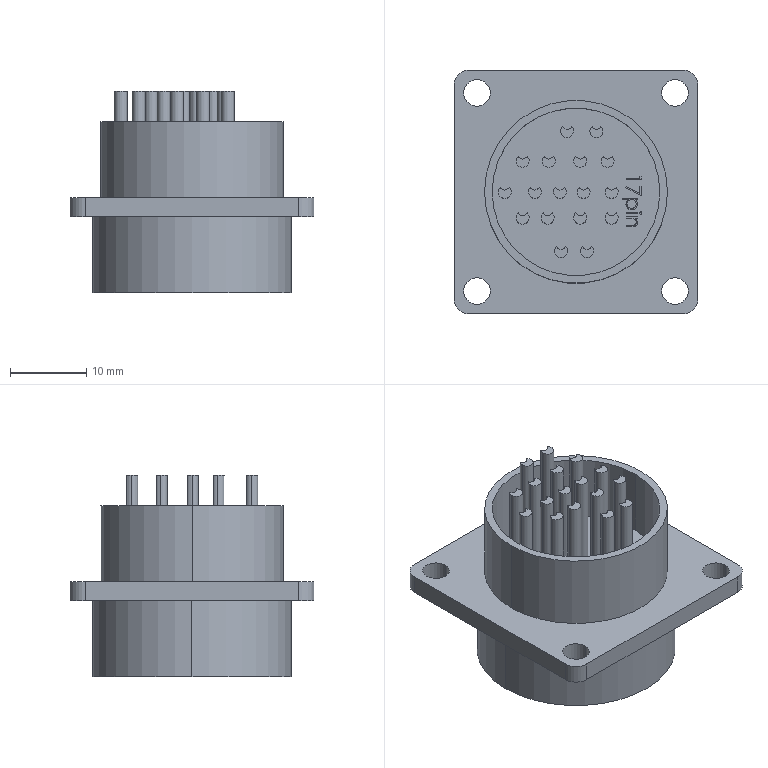Part | NX | features BREP 1 | 1 solid | 290 faces | box 32 x 32 x 26.5 mm | volume 5301 mm3 | plane 136 | cylinder 130 | spline 24 | commonest cylinder face diameters 1.7 x51 1 x35 1.243 x17 3.5 x8 4 x4 24 x4